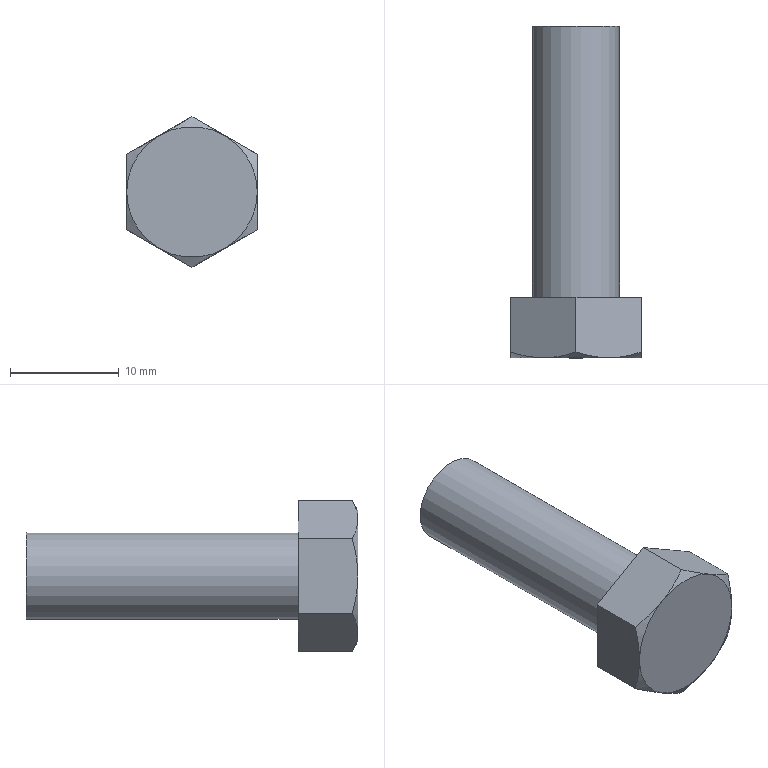Part | NX | features DATUM_CSYS 4, SKETCH 3, EXTRUDE 2, SWP104 1, SYMBOLIC_THREAD 1, UNITE 1 | 1 solid | 16 faces | box 12 x 30.5 x 13.856 mm | volume 1941 mm3 | plane 9 | cone 6 | cylinder 1 | commonest cylinder face diameters 8 x1
STEP:
#1=CARTESIAN_POINT('',(4.,25.,0.));
#2=VERTEX_POINT('',#1);
#3=CARTESIAN_POINT('',(0.,25.,0.));
#4=DIRECTION('',(0.,-1.,0.));
#5=DIRECTION('',(1.,0.,0.));
#6=AXIS2_PLACEMENT_3D('',#3,#4,#5);
#7=CIRCLE('',#6,4.);
#8=EDGE_CURVE('',#2,#2,#7,.T.);
#9=ORIENTED_EDGE('',*,*,#8,.T.);
#10=EDGE_LOOP('',(#9));
#11=FACE_BOUND('',#10,.T.);
#12=CARTESIAN_POINT('',(4.,0.,0.));
#13=VERTEX_POINT('',#12);
#14=CARTESIAN_POINT('',(0.,0.,0.));
#15=DIRECTION('',(0.,-1.,0.));
#16=DIRECTION('',(1.,0.,0.));
#17=AXIS2_PLACEMENT_3D('',#14,#15,#16);
#18=CIRCLE('',#17,4.);
#19=EDGE_CURVE('',#13,#13,#18,.T.);
#20=ORIENTED_EDGE('',*,*,#19,.F.);
#21=EDGE_LOOP('',(#20));
#22=FACE_BOUND('',#21,.T.);
#23=CARTESIAN_POINT('',(0.,25.,0.));
#24=DIRECTION('',(0.,-1.,0.));
#25=DIRECTION('',(0.,0.,-1.));
#26=AXIS2_PLACEMENT_3D('',#23,#24,#25);
#27=CYLINDRICAL_SURFACE('',#26,4.);
#28=ADVANCED_FACE('',(#11,#22),#27,.T.);
#29=ORIENTED_EDGE('',*,*,#8,.F.);
#30=EDGE_LOOP('',(#29));
#31=FACE_BOUND('',#30,.T.);
#32=CARTESIAN_POINT('',(0.,25.,0.));
#33=DIRECTION('',(0.,-1.,0.));
#34=DIRECTION('',(0.,0.,-1.));
#35=AXIS2_PLACEMENT_3D('',#32,#33,#34);
#36=PLANE('',#35);
#37=ADVANCED_FACE('',(#31),#36,.F.);
#38=CARTESIAN_POINT('',(-6.,-4.964,-3.464));
#39=VERTEX_POINT('',#38);
#40=CARTESIAN_POINT('',(-6.,0.,-3.464));
#41=VERTEX_POINT('',#40);
#42=CARTESIAN_POINT('',(-6.,-5.5,-3.464));
#43=DIRECTION('',(0.,1.,0.));
#44=VECTOR('',#43,1000.);
#45=LINE('',#42,#44);
#46=EDGE_CURVE('',#39,#41,#45,.T.);
#47=ORIENTED_EDGE('',*,*,#46,.F.);
#48=CARTESIAN_POINT('',(-6.,-5.5,0.));
#49=VERTEX_POINT('',#48);
#50=CARTESIAN_POINT('',(-6.,-4.964,-3.464));
#51=CARTESIAN_POINT('',(-6.,-5.29,-2.336));
#52=CARTESIAN_POINT('',(-6.,-5.5,-1.172));
#53=CARTESIAN_POINT('',(-6.,-5.5,0.));
#54=B_SPLINE_CURVE_WITH_KNOTS('',3,(#50,#51,#52,#53),.UNSPECIFIED.,.F.,.F.,(4,4),(0.006361,0.009867),.UNSPECIFIED.);
#55=EDGE_CURVE('',#39,#49,#54,.T.);
#56=ORIENTED_EDGE('',*,*,#55,.T.);
#57=CARTESIAN_POINT('',(-6.,-4.964,3.464));
#58=VERTEX_POINT('',#57);
#59=CARTESIAN_POINT('',(-6.,-5.5,0.));
#60=CARTESIAN_POINT('',(-6.,-5.5,1.173));
#61=CARTESIAN_POINT('',(-6.,-5.288,2.344));
#62=CARTESIAN_POINT('',(-6.,-4.964,3.464));
#63=B_SPLINE_CURVE_WITH_KNOTS('',3,(#59,#60,#61,#62),.UNSPECIFIED.,.F.,.F.,(4,4),(0.009867,0.01338),.UNSPECIFIED.);
#64=EDGE_CURVE('',#49,#58,#63,.T.);
#65=ORIENTED_EDGE('',*,*,#64,.T.);
#66=CARTESIAN_POINT('',(-6.,0.,3.464));
#67=VERTEX_POINT('',#66);
#68=CARTESIAN_POINT('',(-6.,-5.5,3.464));
#69=DIRECTION('',(0.,1.,0.));
#70=VECTOR('',#69,1000.);
#71=LINE('',#68,#70);
#72=EDGE_CURVE('',#58,#67,#71,.T.);
#73=ORIENTED_EDGE('',*,*,#72,.T.);
#74=CARTESIAN_POINT('',(-6.,0.,3.464));
#75=DIRECTION('',(0.,0.,-1.));
#76=VECTOR('',#75,1000.);
#77=LINE('',#74,#76);
#78=EDGE_CURVE('',#67,#41,#77,.T.);
#79=ORIENTED_EDGE('',*,*,#78,.T.);
#80=EDGE_LOOP('',(#47,#56,#65,#73,#79));
#81=FACE_BOUND('',#80,.T.);
#82=CARTESIAN_POINT('',(-6.,-5.5,3.464));
#83=DIRECTION('',(1.,0.,0.));
#84=DIRECTION('',(0.,0.,-1.));
#85=AXIS2_PLACEMENT_3D('',#82,#83,#84);
#86=PLANE('',#85);
#87=ADVANCED_FACE('',(#81),#86,.F.);
#88=CARTESIAN_POINT('',(0.,-4.964,-6.928));
#89=VERTEX_POINT('',#88);
#90=CARTESIAN_POINT('',(0.,0.,-6.928));
#91=VERTEX_POINT('',#90);
#92=CARTESIAN_POINT('',(0.,-5.5,-6.928));
#93=DIRECTION('',(0.,1.,0.));
#94=VECTOR('',#93,1000.);
#95=LINE('',#92,#94);
#96=EDGE_CURVE('',#89,#91,#95,.T.);
#97=ORIENTED_EDGE('',*,*,#96,.F.);
#98=CARTESIAN_POINT('',(-3.,-5.5,-5.196));
#99=VERTEX_POINT('',#98);
#100=CARTESIAN_POINT('',(0.,-4.964,-6.928));
#101=CARTESIAN_POINT('',(-0.9815,-5.291,-6.362));
#102=CARTESIAN_POINT('',(-1.978,-5.5,-5.786));
#103=CARTESIAN_POINT('',(-3.,-5.5,-5.196));
#104=B_SPLINE_CURVE_WITH_KNOTS('',3,(#100,#101,#102,#103),.UNSPECIFIED.,.F.,.F.,(4,4),(0.000000238,0.003505),.UNSPECIFIED.);
#105=EDGE_CURVE('',#89,#99,#104,.T.);
#106=ORIENTED_EDGE('',*,*,#105,.T.);
#107=CARTESIAN_POINT('',(-3.,-5.5,-5.196));
#108=CARTESIAN_POINT('',(-4.018,-5.5,-4.608));
#109=CARTESIAN_POINT('',(-5.021,-5.29,-4.029));
#110=CARTESIAN_POINT('',(-6.,-4.964,-3.464));
#111=B_SPLINE_CURVE_WITH_KNOTS('',3,(#107,#108,#109,#110),.UNSPECIFIED.,.F.,.F.,(4,4),(0.003505,0.006997),.UNSPECIFIED.);
#112=EDGE_CURVE('',#99,#39,#111,.T.);
#113=ORIENTED_EDGE('',*,*,#112,.T.);
#114=ORIENTED_EDGE('',*,*,#46,.T.);
#115=CARTESIAN_POINT('',(-6.,0.,-3.464));
#116=DIRECTION('',(0.866,0.,-0.5));
#117=VECTOR('',#116,1000.);
#118=LINE('',#115,#117);
#119=EDGE_CURVE('',#41,#91,#118,.T.);
#120=ORIENTED_EDGE('',*,*,#119,.T.);
#121=EDGE_LOOP('',(#97,#106,#113,#114,#120));
#122=FACE_BOUND('',#121,.T.);
#123=CARTESIAN_POINT('',(-6.,-5.5,-3.464));
#124=DIRECTION('',(0.5,0.,0.866));
#125=DIRECTION('',(0.866,0.,-0.5));
#126=AXIS2_PLACEMENT_3D('',#123,#124,#125);
#127=PLANE('',#126);
#128=ADVANCED_FACE('',(#122),#127,.F.);
#129=CARTESIAN_POINT('',(6.,-4.964,-3.464));
#130=VERTEX_POINT('',#129);
#131=CARTESIAN_POINT('',(6.,0.,-3.464));
#132=VERTEX_POINT('',#131);
#133=CARTESIAN_POINT('',(6.,-5.5,-3.464));
#134=DIRECTION('',(0.,1.,0.));
#135=VECTOR('',#134,1000.);
#136=LINE('',#133,#135);
#137=EDGE_CURVE('',#130,#132,#136,.T.);
#138=ORIENTED_EDGE('',*,*,#137,.F.);
#139=CARTESIAN_POINT('',(3.,-5.5,-5.196));
#140=VERTEX_POINT('',#139);
#141=CARTESIAN_POINT('',(6.,-4.964,-3.464));
#142=CARTESIAN_POINT('',(5.018,-5.291,-4.031));
#143=CARTESIAN_POINT('',(4.022,-5.5,-4.606));
#144=CARTESIAN_POINT('',(3.,-5.5,-5.196));
#145=B_SPLINE_CURVE_WITH_KNOTS('',3,(#141,#142,#143,#144),.UNSPECIFIED.,.F.,.F.,(4,4),(0.000000238,0.003505),.UNSPECIFIED.);
#146=EDGE_CURVE('',#130,#140,#145,.T.);
#147=ORIENTED_EDGE('',*,*,#146,.T.);
#148=CARTESIAN_POINT('',(3.,-5.5,-5.196));
#149=CARTESIAN_POINT('',(1.982,-5.5,-5.784));
#150=CARTESIAN_POINT('',(0.9791,-5.29,-6.363));
#151=CARTESIAN_POINT('',(0.,-4.964,-6.928));
#152=B_SPLINE_CURVE_WITH_KNOTS('',3,(#148,#149,#150,#151),.UNSPECIFIED.,.F.,.F.,(4,4),(0.003505,0.006997),.UNSPECIFIED.);
#153=EDGE_CURVE('',#140,#89,#152,.T.);
#154=ORIENTED_EDGE('',*,*,#153,.T.);
#155=ORIENTED_EDGE('',*,*,#96,.T.);
#156=CARTESIAN_POINT('',(0.,0.,-6.928));
#157=DIRECTION('',(0.866,0.,0.5));
#158=VECTOR('',#157,1000.);
#159=LINE('',#156,#158);
#160=EDGE_CURVE('',#91,#132,#159,.T.);
#161=ORIENTED_EDGE('',*,*,#160,.T.);
#162=EDGE_LOOP('',(#138,#147,#154,#155,#161));
#163=FACE_BOUND('',#162,.T.);
#164=CARTESIAN_POINT('',(0.,-5.5,-6.928));
#165=DIRECTION('',(-0.5,0.,0.866));
#166=DIRECTION('',(0.866,0.,0.5));
#167=AXIS2_PLACEMENT_3D('',#164,#165,#166);
#168=PLANE('',#167);
#169=ADVANCED_FACE('',(#163),#168,.F.);
#170=CARTESIAN_POINT('',(6.,-4.964,3.464));
#171=VERTEX_POINT('',#170);
#172=CARTESIAN_POINT('',(6.,0.,3.464));
#173=VERTEX_POINT('',#172);
#174=CARTESIAN_POINT('',(6.,-5.5,3.464));
#175=DIRECTION('',(0.,1.,0.));
#176=VECTOR('',#175,1000.);
#177=LINE('',#174,#176);
#178=EDGE_CURVE('',#171,#173,#177,.T.);
#179=ORIENTED_EDGE('',*,*,#178,.F.);
#180=CARTESIAN_POINT('',(6.,-5.5,0.));
#181=VERTEX_POINT('',#180);
#182=CARTESIAN_POINT('',(6.,-5.5,0.));
#183=CARTESIAN_POINT('',(6.,-5.5,1.173));
#184=CARTESIAN_POINT('',(6.,-5.288,2.344));
#185=CARTESIAN_POINT('',(6.,-4.964,3.464));
#186=B_SPLINE_CURVE_WITH_KNOTS('',3,(#182,#183,#184,#185),.UNSPECIFIED.,.F.,.F.,(4,4),(0.009867,0.01338),.UNSPECIFIED.);
#187=EDGE_CURVE('',#171,#181,#186,.F.);
#188=ORIENTED_EDGE('',*,*,#187,.T.);
#189=CARTESIAN_POINT('',(6.,-4.964,-3.464));
#190=CARTESIAN_POINT('',(6.,-5.29,-2.336));
#191=CARTESIAN_POINT('',(6.,-5.5,-1.172));
#192=CARTESIAN_POINT('',(6.,-5.5,0.));
#193=B_SPLINE_CURVE_WITH_KNOTS('',3,(#189,#190,#191,#192),.UNSPECIFIED.,.F.,.F.,(4,4),(0.006361,0.009867),.UNSPECIFIED.);
#194=EDGE_CURVE('',#181,#130,#193,.F.);
#195=ORIENTED_EDGE('',*,*,#194,.T.);
#196=ORIENTED_EDGE('',*,*,#137,.T.);
#197=CARTESIAN_POINT('',(6.,0.,-3.464));
#198=DIRECTION('',(0.,0.,1.));
#199=VECTOR('',#198,1000.);
#200=LINE('',#197,#199);
#201=EDGE_CURVE('',#132,#173,#200,.T.);
#202=ORIENTED_EDGE('',*,*,#201,.T.);
#203=EDGE_LOOP('',(#179,#188,#195,#196,#202));
#204=FACE_BOUND('',#203,.T.);
#205=CARTESIAN_POINT('',(6.,-5.5,-3.464));
#206=DIRECTION('',(-1.,0.,0.));
#207=DIRECTION('',(0.,0.,1.));
#208=AXIS2_PLACEMENT_3D('',#205,#206,#207);
#209=PLANE('',#208);
#210=ADVANCED_FACE('',(#204),#209,.F.);
#211=CARTESIAN_POINT('',(0.,-4.964,6.928));
#212=VERTEX_POINT('',#211);
#213=CARTESIAN_POINT('',(0.,0.,6.928));
#214=VERTEX_POINT('',#213);
#215=CARTESIAN_POINT('',(0.,-5.5,6.928));
#216=DIRECTION('',(0.,1.,0.));
#217=VECTOR('',#216,1000.);
#218=LINE('',#215,#217);
#219=EDGE_CURVE('',#212,#214,#218,.T.);
#220=ORIENTED_EDGE('',*,*,#219,.F.);
#221=CARTESIAN_POINT('',(3.,-5.5,5.196));
#222=VERTEX_POINT('',#221);
#223=CARTESIAN_POINT('',(0.,-4.964,6.928));
#224=CARTESIAN_POINT('',(0.9815,-5.291,6.362));
#225=CARTESIAN_POINT('',(1.978,-5.5,5.786));
#226=CARTESIAN_POINT('',(3.,-5.5,5.196));
#227=B_SPLINE_CURVE_WITH_KNOTS('',3,(#223,#224,#225,#226),.UNSPECIFIED.,.F.,.F.,(4,4),(0.000000238,0.003505),.UNSPECIFIED.);
#228=EDGE_CURVE('',#212,#222,#227,.T.);
#229=ORIENTED_EDGE('',*,*,#228,.T.);
#230=CARTESIAN_POINT('',(3.,-5.5,5.196));
#231=CARTESIAN_POINT('',(4.018,-5.5,4.608));
#232=CARTESIAN_POINT('',(5.021,-5.29,4.029));
#233=CARTESIAN_POINT('',(6.,-4.964,3.464));
#234=B_SPLINE_CURVE_WITH_KNOTS('',3,(#230,#231,#232,#233),.UNSPECIFIED.,.F.,.F.,(4,4),(0.003505,0.006997),.UNSPECIFIED.);
#235=EDGE_CURVE('',#222,#171,#234,.T.);
#236=ORIENTED_EDGE('',*,*,#235,.T.);
#237=ORIENTED_EDGE('',*,*,#178,.T.);
#238=CARTESIAN_POINT('',(6.,0.,3.464));
#239=DIRECTION('',(-0.866,0.,0.5));
#240=VECTOR('',#239,1000.);
#241=LINE('',#238,#240);
#242=EDGE_CURVE('',#173,#214,#241,.T.);
#243=ORIENTED_EDGE('',*,*,#242,.T.);
#244=EDGE_LOOP('',(#220,#229,#236,#237,#243));
#245=FACE_BOUND('',#244,.T.);
#246=CARTESIAN_POINT('',(6.,-5.5,3.464));
#247=DIRECTION('',(-0.5,0.,-0.866));
#248=DIRECTION('',(-0.866,0.,0.5));
#249=AXIS2_PLACEMENT_3D('',#246,#247,#248);
#250=PLANE('',#249);
#251=ADVANCED_FACE('',(#245),#250,.F.);
#252=ORIENTED_EDGE('',*,*,#72,.F.);
#253=CARTESIAN_POINT('',(-3.,-5.5,5.196));
#254=VERTEX_POINT('',#253);
#255=CARTESIAN_POINT('',(-6.,-4.964,3.464));
#256=CARTESIAN_POINT('',(-5.018,-5.291,4.031));
#257=CARTESIAN_POINT('',(-4.022,-5.5,4.606));
#258=CARTESIAN_POINT('',(-3.,-5.5,5.196));
#259=B_SPLINE_CURVE_WITH_KNOTS('',3,(#255,#256,#257,#258),.UNSPECIFIED.,.F.,.F.,(4,4),(0.000000238,0.003505),.UNSPECIFIED.);
#260=EDGE_CURVE('',#58,#254,#259,.T.);
#261=ORIENTED_EDGE('',*,*,#260,.T.);
#262=CARTESIAN_POINT('',(-3.,-5.5,5.196));
#263=CARTESIAN_POINT('',(-1.982,-5.5,5.784));
#264=CARTESIAN_POINT('',(-0.9791,-5.29,6.363));
#265=CARTESIAN_POINT('',(0.,-4.964,6.928));
#266=B_SPLINE_CURVE_WITH_KNOTS('',3,(#262,#263,#264,#265),.UNSPECIFIED.,.F.,.F.,(4,4),(0.003505,0.006997),.UNSPECIFIED.);
#267=EDGE_CURVE('',#254,#212,#266,.T.);
#268=ORIENTED_EDGE('',*,*,#267,.T.);
#269=ORIENTED_EDGE('',*,*,#219,.T.);
#270=CARTESIAN_POINT('',(0.,0.,6.928));
#271=DIRECTION('',(-0.866,0.,-0.5));
#272=VECTOR('',#271,1000.);
#273=LINE('',#270,#272);
#274=EDGE_CURVE('',#214,#67,#273,.T.);
#275=ORIENTED_EDGE('',*,*,#274,.T.);
#276=EDGE_LOOP('',(#252,#261,#268,#269,#275));
#277=FACE_BOUND('',#276,.T.);
#278=CARTESIAN_POINT('',(0.,-5.5,6.928));
#279=DIRECTION('',(0.5,0.,-0.866));
#280=DIRECTION('',(-0.866,0.,-0.5));
#281=AXIS2_PLACEMENT_3D('',#278,#279,#280);
#282=PLANE('',#281);
#283=ADVANCED_FACE('',(#277),#282,.F.);
#284=ORIENTED_EDGE('',*,*,#19,.T.);
#285=EDGE_LOOP('',(#284));
#286=FACE_BOUND('',#285,.T.);
#287=ORIENTED_EDGE('',*,*,#78,.F.);
#288=ORIENTED_EDGE('',*,*,#274,.F.);
#289=ORIENTED_EDGE('',*,*,#242,.F.);
#290=ORIENTED_EDGE('',*,*,#201,.F.);
#291=ORIENTED_EDGE('',*,*,#160,.F.);
#292=ORIENTED_EDGE('',*,*,#119,.F.);
#293=EDGE_LOOP('',(#287,#288,#289,#290,#291,#292));
#294=FACE_BOUND('',#293,.T.);
#295=CARTESIAN_POINT('',(0.,0.,0.));
#296=DIRECTION('',(0.,-1.,0.));
#297=DIRECTION('',(0.,0.,-1.));
#298=AXIS2_PLACEMENT_3D('',#295,#296,#297);
#299=PLANE('',#298);
#300=ADVANCED_FACE('',(#286,#294),#299,.F.);
#301=ORIENTED_EDGE('',*,*,#267,.F.);
#302=CARTESIAN_POINT('',(0.,-5.5,0.));
#303=DIRECTION('',(0.,-1.,0.));
#304=DIRECTION('',(0.,0.,-1.));
#305=AXIS2_PLACEMENT_3D('',#302,#303,#304);
#306=CIRCLE('',#305,6.);
#307=EDGE_CURVE('',#222,#254,#306,.T.);
#308=ORIENTED_EDGE('',*,*,#307,.F.);
#309=ORIENTED_EDGE('',*,*,#228,.F.);
#310=EDGE_LOOP('',(#301,#308,#309));
#311=FACE_BOUND('',#310,.T.);
#312=CARTESIAN_POINT('',(0.,-3.8,0.));
#313=DIRECTION('',(0.,1.,0.));
#314=DIRECTION('',(0.,0.,1.));
#315=AXIS2_PLACEMENT_3D('',#312,#313,#314);
#316=CONICAL_SURFACE('',#315,8.944,1.047);
#317=ADVANCED_FACE('',(#311),#316,.T.);
#318=CARTESIAN_POINT('',(0.,-5.5,0.));
#319=DIRECTION('',(0.,-1.,0.));
#320=DIRECTION('',(0.,0.,-1.));
#321=AXIS2_PLACEMENT_3D('',#318,#319,#320);
#322=CIRCLE('',#321,6.);
#323=EDGE_CURVE('',#254,#49,#322,.T.);
#324=ORIENTED_EDGE('',*,*,#323,.F.);
#325=ORIENTED_EDGE('',*,*,#260,.F.);
#326=ORIENTED_EDGE('',*,*,#64,.F.);
#327=EDGE_LOOP('',(#324,#325,#326));
#328=FACE_BOUND('',#327,.T.);
#329=CARTESIAN_POINT('',(0.,-3.8,0.));
#330=DIRECTION('',(0.,1.,0.));
#331=DIRECTION('',(0.,0.,1.));
#332=AXIS2_PLACEMENT_3D('',#329,#330,#331);
#333=CONICAL_SURFACE('',#332,8.944,1.047);
#334=ADVANCED_FACE('',(#328),#333,.T.);
#335=ORIENTED_EDGE('',*,*,#235,.F.);
#336=CARTESIAN_POINT('',(0.,-5.5,0.));
#337=DIRECTION('',(0.,-1.,0.));
#338=DIRECTION('',(0.,0.,-1.));
#339=AXIS2_PLACEMENT_3D('',#336,#337,#338);
#340=CIRCLE('',#339,6.);
#341=EDGE_CURVE('',#181,#222,#340,.T.);
#342=ORIENTED_EDGE('',*,*,#341,.F.);
#343=ORIENTED_EDGE('',*,*,#187,.F.);
#344=EDGE_LOOP('',(#335,#342,#343));
#345=FACE_BOUND('',#344,.T.);
#346=CARTESIAN_POINT('',(0.,-3.8,0.));
#347=DIRECTION('',(0.,1.,0.));
#348=DIRECTION('',(0.,0.,1.));
#349=AXIS2_PLACEMENT_3D('',#346,#347,#348);
#350=CONICAL_SURFACE('',#349,8.944,1.047);
#351=ADVANCED_FACE('',(#345),#350,.T.);
#352=ORIENTED_EDGE('',*,*,#194,.F.);
#353=CARTESIAN_POINT('',(0.,-5.5,0.));
#354=DIRECTION('',(0.,-1.,0.));
#355=DIRECTION('',(0.,0.,-1.));
#356=AXIS2_PLACEMENT_3D('',#353,#354,#355);
#357=CIRCLE('',#356,6.);
#358=EDGE_CURVE('',#140,#181,#357,.T.);
#359=ORIENTED_EDGE('',*,*,#358,.F.);
#360=ORIENTED_EDGE('',*,*,#146,.F.);
#361=EDGE_LOOP('',(#352,#359,#360));
#362=FACE_BOUND('',#361,.T.);
#363=CARTESIAN_POINT('',(0.,-3.8,0.));
#364=DIRECTION('',(0.,1.,0.));
#365=DIRECTION('',(0.,0.,1.));
#366=AXIS2_PLACEMENT_3D('',#363,#364,#365);
#367=CONICAL_SURFACE('',#366,8.944,1.047);
#368=ADVANCED_FACE('',(#362),#367,.T.);
#369=CARTESIAN_POINT('',(0.,-5.5,0.));
#370=DIRECTION('',(0.,-1.,0.));
#371=DIRECTION('',(0.,0.,-1.));
#372=AXIS2_PLACEMENT_3D('',#369,#370,#371);
#373=CIRCLE('',#372,6.);
#374=EDGE_CURVE('',#99,#140,#373,.T.);
#375=ORIENTED_EDGE('',*,*,#374,.F.);
#376=ORIENTED_EDGE('',*,*,#105,.F.);
#377=ORIENTED_EDGE('',*,*,#153,.F.);
#378=EDGE_LOOP('',(#375,#376,#377));
#379=FACE_BOUND('',#378,.T.);
#380=CARTESIAN_POINT('',(0.,-3.8,0.));
#381=DIRECTION('',(0.,1.,0.));
#382=DIRECTION('',(0.,0.,1.));
#383=AXIS2_PLACEMENT_3D('',#380,#381,#382);
#384=CONICAL_SURFACE('',#383,8.944,1.047);
#385=ADVANCED_FACE('',(#379),#384,.T.);
#386=CARTESIAN_POINT('',(0.,-5.5,0.));
#387=DIRECTION('',(0.,-1.,0.));
#388=DIRECTION('',(0.,0.,-1.));
#389=AXIS2_PLACEMENT_3D('',#386,#387,#388);
#390=CIRCLE('',#389,6.);
#391=EDGE_CURVE('',#49,#99,#390,.T.);
#392=ORIENTED_EDGE('',*,*,#391,.F.);
#393=ORIENTED_EDGE('',*,*,#55,.F.);
#394=ORIENTED_EDGE('',*,*,#112,.F.);
#395=EDGE_LOOP('',(#392,#393,#394));
#396=FACE_BOUND('',#395,.T.);
#397=CARTESIAN_POINT('',(0.,-3.8,0.));
#398=DIRECTION('',(0.,1.,0.));
#399=DIRECTION('',(0.,0.,1.));
#400=AXIS2_PLACEMENT_3D('',#397,#398,#399);
#401=CONICAL_SURFACE('',#400,8.944,1.047);
#402=ADVANCED_FACE('',(#396),#401,.T.);
#403=ORIENTED_EDGE('',*,*,#374,.T.);
#404=ORIENTED_EDGE('',*,*,#358,.T.);
#405=ORIENTED_EDGE('',*,*,#341,.T.);
#406=ORIENTED_EDGE('',*,*,#307,.T.);
#407=ORIENTED_EDGE('',*,*,#323,.T.);
#408=ORIENTED_EDGE('',*,*,#391,.T.);
#409=EDGE_LOOP('',(#403,#404,#405,#406,#407,#408));
#410=FACE_BOUND('',#409,.T.);
#411=CARTESIAN_POINT('',(0.,-5.5,0.));
#412=DIRECTION('',(0.,-1.,0.));
#413=DIRECTION('',(0.,0.,-1.));
#414=AXIS2_PLACEMENT_3D('',#411,#412,#413);
#415=PLANE('',#414);
#416=ADVANCED_FACE('',(#410),#415,.T.);
#417=CLOSED_SHELL('',(#28,#37,#87,#128,#169,#210,#251,#283,#300,#317,#334,#351,#368,#385,#402,#416));
#418=MANIFOLD_SOLID_BREP('',#417);
#419=(LENGTH_UNIT()NAMED_UNIT(*)SI_UNIT(.MILLI.,.METRE.));
#420=UNCERTAINTY_MEASURE_WITH_UNIT(LENGTH_MEASURE(0.0508),#419,'','');
#421=(NAMED_UNIT(*)PLANE_ANGLE_UNIT()SI_UNIT($,.RADIAN.));
#422=(NAMED_UNIT(*)SI_UNIT($,.STERADIAN.)SOLID_ANGLE_UNIT());
#423=(GEOMETRIC_REPRESENTATION_CONTEXT(3)GLOBAL_UNCERTAINTY_ASSIGNED_CONTEXT((#420))GLOBAL_UNIT_ASSIGNED_CONTEXT((#419,#421,#422))REPRESENTATION_CONTEXT('',''));
#424=ADVANCED_BREP_SHAPE_REPRESENTATION('',(#418),#423);